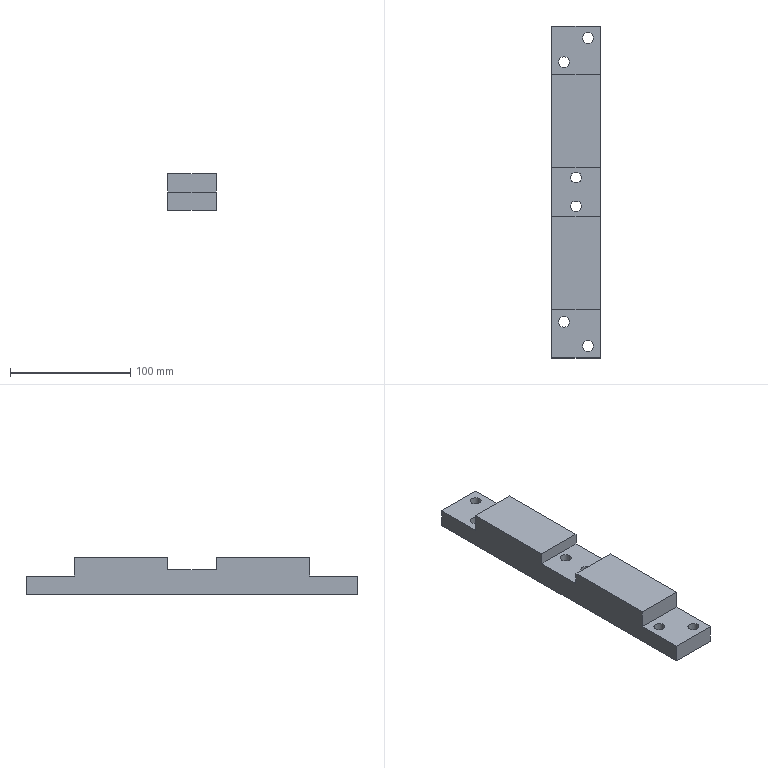Part | NX | features solid 2 | 1 solid | 24 faces | box 40 x 276 x 30 mm | volume 258605 mm3 | plane 16 | cylinder 8 | commonest cylinder face diameters 9 x6 14.5 x2
STEP:
#1=CARTESIAN_POINT('',(3416.5,-108.,-63.5));
#2=VERTEX_POINT('',#1);
#3=CARTESIAN_POINT('',(3421.,-108.,-63.5));
#4=DIRECTION('',(0.,0.,-1.));
#5=DIRECTION('',(-1.,0.,0.));
#6=AXIS2_PLACEMENT_3D('',#3,#4,#5);
#7=CIRCLE('',#6,4.5);
#8=EDGE_CURVE('',#2,#2,#7,.T.);
#9=ORIENTED_EDGE('',*,*,#8,.F.);
#10=EDGE_LOOP('',(#9));
#11=FACE_BOUND('',#10,.T.);
#12=CARTESIAN_POINT('',(3438.25,-12.,-63.5));
#13=VERTEX_POINT('',#12);
#14=CARTESIAN_POINT('',(3431.,-12.,-63.5));
#15=DIRECTION('',(0.,0.,1.));
#16=DIRECTION('',(1.,0.,0.));
#17=AXIS2_PLACEMENT_3D('',#14,#15,#16);
#18=CIRCLE('',#17,7.25);
#19=EDGE_CURVE('',#13,#13,#18,.T.);
#20=ORIENTED_EDGE('',*,*,#19,.T.);
#21=EDGE_LOOP('',(#20));
#22=FACE_BOUND('',#21,.T.);
#23=CARTESIAN_POINT('',(3411.,138.,-63.5));
#24=VERTEX_POINT('',#23);
#25=CARTESIAN_POINT('',(3411.,-138.,-63.5));
#26=VERTEX_POINT('',#25);
#27=CARTESIAN_POINT('',(3411.,0.,-63.5));
#28=DIRECTION('',(0.,-1.,0.));
#29=VECTOR('',#28,1000.);
#30=LINE('',#27,#29);
#31=EDGE_CURVE('',#24,#26,#30,.T.);
#32=ORIENTED_EDGE('',*,*,#31,.F.);
#33=CARTESIAN_POINT('',(3451.,138.,-63.5));
#34=VERTEX_POINT('',#33);
#35=CARTESIAN_POINT('',(3699.,138.,-63.5));
#36=DIRECTION('',(1.,0.,0.));
#37=VECTOR('',#36,1000.);
#38=LINE('',#35,#37);
#39=EDGE_CURVE('',#24,#34,#38,.T.);
#40=ORIENTED_EDGE('',*,*,#39,.T.);
#41=CARTESIAN_POINT('',(3451.,-138.,-63.5));
#42=VERTEX_POINT('',#41);
#43=CARTESIAN_POINT('',(3451.,0.,-63.5));
#44=DIRECTION('',(0.,1.,0.));
#45=VECTOR('',#44,1000.);
#46=LINE('',#43,#45);
#47=EDGE_CURVE('',#42,#34,#46,.T.);
#48=ORIENTED_EDGE('',*,*,#47,.F.);
#49=CARTESIAN_POINT('',(3699.,-138.,-63.5));
#50=DIRECTION('',(1.,0.,0.));
#51=VECTOR('',#50,1000.);
#52=LINE('',#49,#51);
#53=EDGE_CURVE('',#26,#42,#52,.T.);
#54=ORIENTED_EDGE('',*,*,#53,.F.);
#55=EDGE_LOOP('',(#32,#40,#48,#54));
#56=FACE_BOUND('',#55,.T.);
#57=CARTESIAN_POINT('',(3445.5,-128.,-63.5));
#58=VERTEX_POINT('',#57);
#59=CARTESIAN_POINT('',(3441.,-128.,-63.5));
#60=DIRECTION('',(0.,0.,1.));
#61=DIRECTION('',(1.,0.,0.));
#62=AXIS2_PLACEMENT_3D('',#59,#60,#61);
#63=CIRCLE('',#62,4.5);
#64=EDGE_CURVE('',#58,#58,#63,.T.);
#65=ORIENTED_EDGE('',*,*,#64,.T.);
#66=EDGE_LOOP('',(#65));
#67=FACE_BOUND('',#66,.T.);
#68=CARTESIAN_POINT('',(3416.5,108.,-63.5));
#69=VERTEX_POINT('',#68);
#70=CARTESIAN_POINT('',(3421.,108.,-63.5));
#71=DIRECTION('',(0.,0.,1.));
#72=DIRECTION('',(-1.,0.,0.));
#73=AXIS2_PLACEMENT_3D('',#70,#71,#72);
#74=CIRCLE('',#73,4.5);
#75=EDGE_CURVE('',#69,#69,#74,.T.);
#76=ORIENTED_EDGE('',*,*,#75,.T.);
#77=EDGE_LOOP('',(#76));
#78=FACE_BOUND('',#77,.T.);
#79=CARTESIAN_POINT('',(3438.25,12.,-63.5));
#80=VERTEX_POINT('',#79);
#81=CARTESIAN_POINT('',(3431.,12.,-63.5));
#82=DIRECTION('',(0.,0.,-1.));
#83=DIRECTION('',(1.,0.,0.));
#84=AXIS2_PLACEMENT_3D('',#81,#82,#83);
#85=CIRCLE('',#84,7.25);
#86=EDGE_CURVE('',#80,#80,#85,.T.);
#87=ORIENTED_EDGE('',*,*,#86,.F.);
#88=EDGE_LOOP('',(#87));
#89=FACE_BOUND('',#88,.T.);
#90=CARTESIAN_POINT('',(3445.5,128.,-63.5));
#91=VERTEX_POINT('',#90);
#92=CARTESIAN_POINT('',(3441.,128.,-63.5));
#93=DIRECTION('',(0.,0.,-1.));
#94=DIRECTION('',(1.,0.,0.));
#95=AXIS2_PLACEMENT_3D('',#92,#93,#94);
#96=CIRCLE('',#95,4.5);
#97=EDGE_CURVE('',#91,#91,#96,.T.);
#98=ORIENTED_EDGE('',*,*,#97,.F.);
#99=EDGE_LOOP('',(#98));
#100=FACE_BOUND('',#99,.T.);
#101=CARTESIAN_POINT('',(3421.,0.,-63.5));
#102=DIRECTION('',(0.,0.,-1.));
#103=DIRECTION('',(1.,0.,0.));
#104=AXIS2_PLACEMENT_3D('',#101,#102,#103);
#105=PLANE('',#104);
#106=ADVANCED_FACE('',(#11,#22,#56,#67,#78,#89,#100),#105,.T.);
#107=CARTESIAN_POINT('',(3411.,20.,-43.5));
#108=VERTEX_POINT('',#107);
#109=CARTESIAN_POINT('',(3411.,-20.,-43.5));
#110=VERTEX_POINT('',#109);
#111=CARTESIAN_POINT('',(3411.,0.,-43.5));
#112=DIRECTION('',(0.,-1.,0.));
#113=VECTOR('',#112,1000.);
#114=LINE('',#111,#113);
#115=EDGE_CURVE('',#108,#110,#114,.T.);
#116=ORIENTED_EDGE('',*,*,#115,.F.);
#117=CARTESIAN_POINT('',(3411.,20.,-33.5));
#118=VERTEX_POINT('',#117);
#119=CARTESIAN_POINT('',(3411.,20.,-63.5));
#120=DIRECTION('',(0.,0.,1.));
#121=VECTOR('',#120,1000.);
#122=LINE('',#119,#121);
#123=EDGE_CURVE('',#108,#118,#122,.T.);
#124=ORIENTED_EDGE('',*,*,#123,.T.);
#125=CARTESIAN_POINT('',(3411.,98.,-33.5));
#126=VERTEX_POINT('',#125);
#127=CARTESIAN_POINT('',(3411.,0.,-33.5));
#128=DIRECTION('',(0.,-1.,0.));
#129=VECTOR('',#128,1000.);
#130=LINE('',#127,#129);
#131=EDGE_CURVE('',#126,#118,#130,.T.);
#132=ORIENTED_EDGE('',*,*,#131,.F.);
#133=CARTESIAN_POINT('',(3411.,98.,-48.5));
#134=VERTEX_POINT('',#133);
#135=CARTESIAN_POINT('',(3411.,98.,-53.5));
#136=DIRECTION('',(0.,0.,1.));
#137=VECTOR('',#136,1000.);
#138=LINE('',#135,#137);
#139=EDGE_CURVE('',#134,#126,#138,.T.);
#140=ORIENTED_EDGE('',*,*,#139,.F.);
#141=CARTESIAN_POINT('',(3411.,138.,-48.5));
#142=VERTEX_POINT('',#141);
#143=CARTESIAN_POINT('',(3411.,0.,-48.5));
#144=DIRECTION('',(0.,1.,0.));
#145=VECTOR('',#144,1000.);
#146=LINE('',#143,#145);
#147=EDGE_CURVE('',#134,#142,#146,.T.);
#148=ORIENTED_EDGE('',*,*,#147,.T.);
#149=CARTESIAN_POINT('',(3411.,138.,-63.5));
#150=DIRECTION('',(0.,0.,1.));
#151=VECTOR('',#150,1000.);
#152=LINE('',#149,#151);
#153=EDGE_CURVE('',#24,#142,#152,.T.);
#154=ORIENTED_EDGE('',*,*,#153,.F.);
#155=ORIENTED_EDGE('',*,*,#31,.T.);
#156=CARTESIAN_POINT('',(3411.,-138.,-48.5));
#157=VERTEX_POINT('',#156);
#158=CARTESIAN_POINT('',(3411.,-138.,-63.5));
#159=DIRECTION('',(0.,0.,1.));
#160=VECTOR('',#159,1000.);
#161=LINE('',#158,#160);
#162=EDGE_CURVE('',#26,#157,#161,.T.);
#163=ORIENTED_EDGE('',*,*,#162,.T.);
#164=CARTESIAN_POINT('',(3411.,-98.,-48.5));
#165=VERTEX_POINT('',#164);
#166=CARTESIAN_POINT('',(3411.,0.,-48.5));
#167=DIRECTION('',(0.,-1.,0.));
#168=VECTOR('',#167,1000.);
#169=LINE('',#166,#168);
#170=EDGE_CURVE('',#165,#157,#169,.T.);
#171=ORIENTED_EDGE('',*,*,#170,.F.);
#172=CARTESIAN_POINT('',(3411.,-98.,-33.5));
#173=VERTEX_POINT('',#172);
#174=CARTESIAN_POINT('',(3411.,-98.,-53.5));
#175=DIRECTION('',(0.,0.,1.));
#176=VECTOR('',#175,1000.);
#177=LINE('',#174,#176);
#178=EDGE_CURVE('',#165,#173,#177,.T.);
#179=ORIENTED_EDGE('',*,*,#178,.T.);
#180=CARTESIAN_POINT('',(3411.,-20.,-33.5));
#181=VERTEX_POINT('',#180);
#182=CARTESIAN_POINT('',(3411.,0.,-33.5));
#183=DIRECTION('',(0.,1.,0.));
#184=VECTOR('',#183,1000.);
#185=LINE('',#182,#184);
#186=EDGE_CURVE('',#173,#181,#185,.T.);
#187=ORIENTED_EDGE('',*,*,#186,.T.);
#188=CARTESIAN_POINT('',(3411.,-20.,-63.5));
#189=DIRECTION('',(0.,0.,1.));
#190=VECTOR('',#189,1000.);
#191=LINE('',#188,#190);
#192=EDGE_CURVE('',#110,#181,#191,.T.);
#193=ORIENTED_EDGE('',*,*,#192,.F.);
#194=EDGE_LOOP('',(#116,#124,#132,#140,#148,#154,#155,#163,#171,#179,#187,#193));
#195=FACE_BOUND('',#194,.T.);
#196=CARTESIAN_POINT('',(3411.,0.,-63.5));
#197=DIRECTION('',(-1.,0.,0.));
#198=DIRECTION('',(0.,0.,-1.));
#199=AXIS2_PLACEMENT_3D('',#196,#197,#198);
#200=PLANE('',#199);
#201=ADVANCED_FACE('',(#195),#200,.T.);
#202=ORIENTED_EDGE('',*,*,#47,.T.);
#203=CARTESIAN_POINT('',(3451.,138.,-48.5));
#204=VERTEX_POINT('',#203);
#205=CARTESIAN_POINT('',(3451.,138.,-53.5));
#206=DIRECTION('',(0.,0.,1.));
#207=VECTOR('',#206,1000.);
#208=LINE('',#205,#207);
#209=EDGE_CURVE('',#34,#204,#208,.T.);
#210=ORIENTED_EDGE('',*,*,#209,.T.);
#211=CARTESIAN_POINT('',(3451.,98.,-48.5));
#212=VERTEX_POINT('',#211);
#213=CARTESIAN_POINT('',(3451.,0.,-48.5));
#214=DIRECTION('',(0.,-1.,0.));
#215=VECTOR('',#214,1000.);
#216=LINE('',#213,#215);
#217=EDGE_CURVE('',#204,#212,#216,.T.);
#218=ORIENTED_EDGE('',*,*,#217,.T.);
#219=CARTESIAN_POINT('',(3451.,98.,-33.5));
#220=VERTEX_POINT('',#219);
#221=CARTESIAN_POINT('',(3451.,98.,-63.5));
#222=DIRECTION('',(0.,0.,1.));
#223=VECTOR('',#222,1000.);
#224=LINE('',#221,#223);
#225=EDGE_CURVE('',#212,#220,#224,.T.);
#226=ORIENTED_EDGE('',*,*,#225,.T.);
#227=CARTESIAN_POINT('',(3451.,20.,-33.5));
#228=VERTEX_POINT('',#227);
#229=CARTESIAN_POINT('',(3451.,0.,-33.5));
#230=DIRECTION('',(0.,1.,0.));
#231=VECTOR('',#230,1000.);
#232=LINE('',#229,#231);
#233=EDGE_CURVE('',#228,#220,#232,.T.);
#234=ORIENTED_EDGE('',*,*,#233,.F.);
#235=CARTESIAN_POINT('',(3451.,20.,-43.5));
#236=VERTEX_POINT('',#235);
#237=CARTESIAN_POINT('',(3451.,20.,-63.5));
#238=DIRECTION('',(0.,0.,-1.));
#239=VECTOR('',#238,1000.);
#240=LINE('',#237,#239);
#241=EDGE_CURVE('',#228,#236,#240,.T.);
#242=ORIENTED_EDGE('',*,*,#241,.T.);
#243=CARTESIAN_POINT('',(3451.,-20.,-43.5));
#244=VERTEX_POINT('',#243);
#245=CARTESIAN_POINT('',(3451.,0.,-43.5));
#246=DIRECTION('',(0.,1.,0.));
#247=VECTOR('',#246,1000.);
#248=LINE('',#245,#247);
#249=EDGE_CURVE('',#244,#236,#248,.T.);
#250=ORIENTED_EDGE('',*,*,#249,.F.);
#251=CARTESIAN_POINT('',(3451.,-20.,-33.5));
#252=VERTEX_POINT('',#251);
#253=CARTESIAN_POINT('',(3451.,-20.,-63.5));
#254=DIRECTION('',(0.,0.,-1.));
#255=VECTOR('',#254,1000.);
#256=LINE('',#253,#255);
#257=EDGE_CURVE('',#252,#244,#256,.T.);
#258=ORIENTED_EDGE('',*,*,#257,.F.);
#259=CARTESIAN_POINT('',(3451.,-98.,-33.5));
#260=VERTEX_POINT('',#259);
#261=CARTESIAN_POINT('',(3451.,0.,-33.5));
#262=DIRECTION('',(0.,-1.,0.));
#263=VECTOR('',#262,1000.);
#264=LINE('',#261,#263);
#265=EDGE_CURVE('',#252,#260,#264,.T.);
#266=ORIENTED_EDGE('',*,*,#265,.T.);
#267=CARTESIAN_POINT('',(3451.,-98.,-48.5));
#268=VERTEX_POINT('',#267);
#269=CARTESIAN_POINT('',(3451.,-98.,-63.5));
#270=DIRECTION('',(0.,0.,1.));
#271=VECTOR('',#270,1000.);
#272=LINE('',#269,#271);
#273=EDGE_CURVE('',#268,#260,#272,.T.);
#274=ORIENTED_EDGE('',*,*,#273,.F.);
#275=CARTESIAN_POINT('',(3451.,-138.,-48.5));
#276=VERTEX_POINT('',#275);
#277=CARTESIAN_POINT('',(3451.,0.,-48.5));
#278=DIRECTION('',(0.,1.,0.));
#279=VECTOR('',#278,1000.);
#280=LINE('',#277,#279);
#281=EDGE_CURVE('',#276,#268,#280,.T.);
#282=ORIENTED_EDGE('',*,*,#281,.F.);
#283=CARTESIAN_POINT('',(3451.,-138.,-53.5));
#284=DIRECTION('',(0.,0.,1.));
#285=VECTOR('',#284,1000.);
#286=LINE('',#283,#285);
#287=EDGE_CURVE('',#42,#276,#286,.T.);
#288=ORIENTED_EDGE('',*,*,#287,.F.);
#289=EDGE_LOOP('',(#202,#210,#218,#226,#234,#242,#250,#258,#266,#274,#282,#288));
#290=FACE_BOUND('',#289,.T.);
#291=CARTESIAN_POINT('',(3451.,0.,-63.5));
#292=DIRECTION('',(1.,0.,0.));
#293=DIRECTION('',(0.,0.,1.));
#294=AXIS2_PLACEMENT_3D('',#291,#292,#293);
#295=PLANE('',#294);
#296=ADVANCED_FACE('',(#290),#295,.T.);
#297=CARTESIAN_POINT('',(3435.5,-12.,-43.5));
#298=VERTEX_POINT('',#297);
#299=CARTESIAN_POINT('',(3431.,-12.,-43.5));
#300=DIRECTION('',(0.,0.,-1.));
#301=DIRECTION('',(1.,0.,0.));
#302=AXIS2_PLACEMENT_3D('',#299,#300,#301);
#303=CIRCLE('',#302,4.5);
#304=EDGE_CURVE('',#298,#298,#303,.T.);
#305=ORIENTED_EDGE('',*,*,#304,.T.);
#306=EDGE_LOOP('',(#305));
#307=FACE_BOUND('',#306,.T.);
#308=ORIENTED_EDGE('',*,*,#249,.T.);
#309=CARTESIAN_POINT('',(2860.,20.,-43.5));
#310=DIRECTION('',(-1.,0.,0.));
#311=VECTOR('',#310,1000.);
#312=LINE('',#309,#311);
#313=EDGE_CURVE('',#236,#108,#312,.T.);
#314=ORIENTED_EDGE('',*,*,#313,.T.);
#315=ORIENTED_EDGE('',*,*,#115,.T.);
#316=CARTESIAN_POINT('',(2860.,-20.,-43.5));
#317=DIRECTION('',(-1.,0.,0.));
#318=VECTOR('',#317,1000.);
#319=LINE('',#316,#318);
#320=EDGE_CURVE('',#244,#110,#319,.T.);
#321=ORIENTED_EDGE('',*,*,#320,.F.);
#322=EDGE_LOOP('',(#308,#314,#315,#321));
#323=FACE_BOUND('',#322,.T.);
#324=CARTESIAN_POINT('',(3435.5,12.,-43.5));
#325=VERTEX_POINT('',#324);
#326=CARTESIAN_POINT('',(3431.,12.,-43.5));
#327=DIRECTION('',(0.,0.,1.));
#328=DIRECTION('',(1.,0.,0.));
#329=AXIS2_PLACEMENT_3D('',#326,#327,#328);
#330=CIRCLE('',#329,4.5);
#331=EDGE_CURVE('',#325,#325,#330,.T.);
#332=ORIENTED_EDGE('',*,*,#331,.F.);
#333=EDGE_LOOP('',(#332));
#334=FACE_BOUND('',#333,.T.);
#335=CARTESIAN_POINT('',(2544.879,0.,-43.5));
#336=DIRECTION('',(0.,0.,1.));
#337=DIRECTION('',(-1.,0.,0.));
#338=AXIS2_PLACEMENT_3D('',#335,#336,#337);
#339=PLANE('',#338);
#340=ADVANCED_FACE('',(#307,#323,#334),#339,.T.);
#341=CARTESIAN_POINT('',(3421.,-20.,-33.5));
#342=DIRECTION('',(1.,0.,0.));
#343=VECTOR('',#342,1000.);
#344=LINE('',#341,#343);
#345=EDGE_CURVE('',#181,#252,#344,.T.);
#346=ORIENTED_EDGE('',*,*,#345,.F.);
#347=ORIENTED_EDGE('',*,*,#186,.F.);
#348=CARTESIAN_POINT('',(3699.,-98.,-33.5));
#349=DIRECTION('',(1.,0.,0.));
#350=VECTOR('',#349,1000.);
#351=LINE('',#348,#350);
#352=EDGE_CURVE('',#173,#260,#351,.T.);
#353=ORIENTED_EDGE('',*,*,#352,.T.);
#354=ORIENTED_EDGE('',*,*,#265,.F.);
#355=EDGE_LOOP('',(#346,#347,#353,#354));
#356=FACE_BOUND('',#355,.T.);
#357=CARTESIAN_POINT('',(3421.,0.,-33.5));
#358=DIRECTION('',(0.,0.,1.));
#359=DIRECTION('',(-1.,0.,0.));
#360=AXIS2_PLACEMENT_3D('',#357,#358,#359);
#361=PLANE('',#360);
#362=ADVANCED_FACE('',(#356),#361,.T.);
#363=CARTESIAN_POINT('',(3699.,-138.,-48.5));
#364=DIRECTION('',(1.,0.,0.));
#365=VECTOR('',#364,1000.);
#366=LINE('',#363,#365);
#367=EDGE_CURVE('',#157,#276,#366,.T.);
#368=ORIENTED_EDGE('',*,*,#367,.F.);
#369=ORIENTED_EDGE('',*,*,#162,.F.);
#370=ORIENTED_EDGE('',*,*,#53,.T.);
#371=ORIENTED_EDGE('',*,*,#287,.T.);
#372=EDGE_LOOP('',(#368,#369,#370,#371));
#373=FACE_BOUND('',#372,.T.);
#374=CARTESIAN_POINT('',(3699.,-138.,-53.5));
#375=DIRECTION('',(0.,-1.,0.));
#376=DIRECTION('',(0.,0.,1.));
#377=AXIS2_PLACEMENT_3D('',#374,#375,#376);
#378=PLANE('',#377);
#379=ADVANCED_FACE('',(#373),#378,.T.);
#380=CARTESIAN_POINT('',(3445.5,-128.,-48.5));
#381=VERTEX_POINT('',#380);
#382=CARTESIAN_POINT('',(3441.,-128.,-48.5));
#383=DIRECTION('',(0.,0.,1.));
#384=DIRECTION('',(1.,0.,0.));
#385=AXIS2_PLACEMENT_3D('',#382,#383,#384);
#386=CIRCLE('',#385,4.5);
#387=EDGE_CURVE('',#381,#381,#386,.T.);
#388=ORIENTED_EDGE('',*,*,#387,.F.);
#389=EDGE_LOOP('',(#388));
#390=FACE_BOUND('',#389,.T.);
#391=CARTESIAN_POINT('',(3425.5,-108.,-48.5));
#392=VERTEX_POINT('',#391);
#393=CARTESIAN_POINT('',(3421.,-108.,-48.5));
#394=DIRECTION('',(0.,0.,1.));
#395=DIRECTION('',(1.,0.,0.));
#396=AXIS2_PLACEMENT_3D('',#393,#394,#395);
#397=CIRCLE('',#396,4.5);
#398=EDGE_CURVE('',#392,#392,#397,.T.);
#399=ORIENTED_EDGE('',*,*,#398,.F.);
#400=EDGE_LOOP('',(#399));
#401=FACE_BOUND('',#400,.T.);
#402=ORIENTED_EDGE('',*,*,#281,.T.);
#403=CARTESIAN_POINT('',(3699.,-98.,-48.5));
#404=DIRECTION('',(-1.,0.,0.));
#405=VECTOR('',#404,1000.);
#406=LINE('',#403,#405);
#407=EDGE_CURVE('',#268,#165,#406,.T.);
#408=ORIENTED_EDGE('',*,*,#407,.T.);
#409=ORIENTED_EDGE('',*,*,#170,.T.);
#410=ORIENTED_EDGE('',*,*,#367,.T.);
#411=EDGE_LOOP('',(#402,#408,#409,#410));
#412=FACE_BOUND('',#411,.T.);
#413=CARTESIAN_POINT('',(3411.,-138.,-48.5));
#414=DIRECTION('',(0.,0.,1.));
#415=DIRECTION('',(-1.,0.,0.));
#416=AXIS2_PLACEMENT_3D('',#413,#414,#415);
#417=PLANE('',#416);
#418=ADVANCED_FACE('',(#390,#401,#412),#417,.T.);
#419=ORIENTED_EDGE('',*,*,#273,.T.);
#420=ORIENTED_EDGE('',*,*,#352,.F.);
#421=ORIENTED_EDGE('',*,*,#178,.F.);
#422=ORIENTED_EDGE('',*,*,#407,.F.);
#423=EDGE_LOOP('',(#419,#420,#421,#422));
#424=FACE_BOUND('',#423,.T.);
#425=CARTESIAN_POINT('',(3699.,-98.,-53.5));
#426=DIRECTION('',(0.,1.,0.));
#427=DIRECTION('',(0.,0.,-1.));
#428=AXIS2_PLACEMENT_3D('',#425,#426,#427);
#429=PLANE('',#428);
#430=ADVANCED_FACE('',(#424),#429,.F.);
#431=ORIENTED_EDGE('',*,*,#192,.T.);
#432=ORIENTED_EDGE('',*,*,#345,.T.);
#433=ORIENTED_EDGE('',*,*,#257,.T.);
#434=ORIENTED_EDGE('',*,*,#320,.T.);
#435=EDGE_LOOP('',(#431,#432,#433,#434));
#436=FACE_BOUND('',#435,.T.);
#437=CARTESIAN_POINT('',(2860.,-20.,-23.5));
#438=DIRECTION('',(0.,-1.,0.));
#439=DIRECTION('',(0.,0.,1.));
#440=AXIS2_PLACEMENT_3D('',#437,#438,#439);
#441=PLANE('',#440);
#442=ADVANCED_FACE('',(#436),#441,.F.);
#443=CARTESIAN_POINT('',(3435.5,-12.,-52.5));
#444=VERTEX_POINT('',#443);
#445=CARTESIAN_POINT('',(3431.,-12.,-52.5));
#446=DIRECTION('',(0.,0.,1.));
#447=DIRECTION('',(1.,0.,0.));
#448=AXIS2_PLACEMENT_3D('',#445,#446,#447);
#449=CIRCLE('',#448,4.5);
#450=EDGE_CURVE('',#444,#444,#449,.T.);
#451=ORIENTED_EDGE('',*,*,#450,.F.);
#452=EDGE_LOOP('',(#451));
#453=FACE_BOUND('',#452,.T.);
#454=ORIENTED_EDGE('',*,*,#304,.F.);
#455=EDGE_LOOP('',(#454));
#456=FACE_BOUND('',#455,.T.);
#457=CARTESIAN_POINT('',(3431.,-12.,-63.5));
#458=DIRECTION('',(0.,0.,1.));
#459=DIRECTION('',(-1.,0.,0.));
#460=AXIS2_PLACEMENT_3D('',#457,#458,#459);
#461=CYLINDRICAL_SURFACE('',#460,4.5);
#462=ADVANCED_FACE('',(#453,#456),#461,.F.);
#463=ORIENTED_EDGE('',*,*,#450,.T.);
#464=EDGE_LOOP('',(#463));
#465=FACE_BOUND('',#464,.T.);
#466=CARTESIAN_POINT('',(3438.25,-12.,-52.5));
#467=VERTEX_POINT('',#466);
#468=CARTESIAN_POINT('',(3431.,-12.,-52.5));
#469=DIRECTION('',(0.,0.,1.));
#470=DIRECTION('',(1.,0.,0.));
#471=AXIS2_PLACEMENT_3D('',#468,#469,#470);
#472=CIRCLE('',#471,7.25);
#473=EDGE_CURVE('',#467,#467,#472,.T.);
#474=ORIENTED_EDGE('',*,*,#473,.F.);
#475=EDGE_LOOP('',(#474));
#476=FACE_BOUND('',#475,.T.);
#477=CARTESIAN_POINT('',(3431.,-12.,-52.5));
#478=DIRECTION('',(0.,0.,1.));
#479=DIRECTION('',(-1.,0.,0.));
#480=AXIS2_PLACEMENT_3D('',#477,#478,#479);
#481=PLANE('',#480);
#482=ADVANCED_FACE('',(#465,#476),#481,.F.);
#483=ORIENTED_EDGE('',*,*,#473,.T.);
#484=EDGE_LOOP('',(#483));
#485=FACE_BOUND('',#484,.T.);
#486=ORIENTED_EDGE('',*,*,#19,.F.);
#487=EDGE_LOOP('',(#486));
#488=FACE_BOUND('',#487,.T.);
#489=CARTESIAN_POINT('',(3431.,-12.,-63.5));
#490=DIRECTION('',(0.,0.,1.));
#491=DIRECTION('',(-1.,0.,0.));
#492=AXIS2_PLACEMENT_3D('',#489,#490,#491);
#493=CYLINDRICAL_SURFACE('',#492,7.25);
#494=ADVANCED_FACE('',(#485,#488),#493,.F.);
#495=ORIENTED_EDGE('',*,*,#398,.T.);
#496=EDGE_LOOP('',(#495));
#497=FACE_BOUND('',#496,.T.);
#498=ORIENTED_EDGE('',*,*,#8,.T.);
#499=EDGE_LOOP('',(#498));
#500=FACE_BOUND('',#499,.T.);
#501=CARTESIAN_POINT('',(3421.,-108.,-74.5));
#502=DIRECTION('',(0.,0.,1.));
#503=DIRECTION('',(-1.,0.,0.));
#504=AXIS2_PLACEMENT_3D('',#501,#502,#503);
#505=CYLINDRICAL_SURFACE('',#504,4.5);
#506=ADVANCED_FACE('',(#497,#500),#505,.F.);
#507=ORIENTED_EDGE('',*,*,#387,.T.);
#508=EDGE_LOOP('',(#507));
#509=FACE_BOUND('',#508,.T.);
#510=ORIENTED_EDGE('',*,*,#64,.F.);
#511=EDGE_LOOP('',(#510));
#512=FACE_BOUND('',#511,.T.);
#513=CARTESIAN_POINT('',(3441.,-128.,-74.5));
#514=DIRECTION('',(0.,0.,1.));
#515=DIRECTION('',(1.,0.,0.));
#516=AXIS2_PLACEMENT_3D('',#513,#514,#515);
#517=CYLINDRICAL_SURFACE('',#516,4.5);
#518=ADVANCED_FACE('',(#509,#512),#517,.F.);
#519=CARTESIAN_POINT('',(3421.,20.,-33.5));
#520=DIRECTION('',(1.,0.,0.));
#521=VECTOR('',#520,1000.);
#522=LINE('',#519,#521);
#523=EDGE_CURVE('',#118,#228,#522,.T.);
#524=ORIENTED_EDGE('',*,*,#523,.T.);
#525=ORIENTED_EDGE('',*,*,#233,.T.);
#526=CARTESIAN_POINT('',(3699.,98.,-33.5));
#527=DIRECTION('',(1.,0.,0.));
#528=VECTOR('',#527,1000.);
#529=LINE('',#526,#528);
#530=EDGE_CURVE('',#126,#220,#529,.T.);
#531=ORIENTED_EDGE('',*,*,#530,.F.);
#532=ORIENTED_EDGE('',*,*,#131,.T.);
#533=EDGE_LOOP('',(#524,#525,#531,#532));
#534=FACE_BOUND('',#533,.T.);
#535=CARTESIAN_POINT('',(3421.,0.,-33.5));
#536=DIRECTION('',(0.,0.,1.));
#537=DIRECTION('',(-1.,0.,0.));
#538=AXIS2_PLACEMENT_3D('',#535,#536,#537);
#539=PLANE('',#538);
#540=ADVANCED_FACE('',(#534),#539,.T.);
#541=CARTESIAN_POINT('',(3699.,138.,-48.5));
#542=DIRECTION('',(1.,0.,0.));
#543=VECTOR('',#542,1000.);
#544=LINE('',#541,#543);
#545=EDGE_CURVE('',#142,#204,#544,.T.);
#546=ORIENTED_EDGE('',*,*,#545,.T.);
#547=ORIENTED_EDGE('',*,*,#209,.F.);
#548=ORIENTED_EDGE('',*,*,#39,.F.);
#549=ORIENTED_EDGE('',*,*,#153,.T.);
#550=EDGE_LOOP('',(#546,#547,#548,#549));
#551=FACE_BOUND('',#550,.T.);
#552=CARTESIAN_POINT('',(3699.,138.,-53.5));
#553=DIRECTION('',(0.,1.,0.));
#554=DIRECTION('',(0.,0.,1.));
#555=AXIS2_PLACEMENT_3D('',#552,#553,#554);
#556=PLANE('',#555);
#557=ADVANCED_FACE('',(#551),#556,.T.);
#558=CARTESIAN_POINT('',(3445.5,128.,-48.5));
#559=VERTEX_POINT('',#558);
#560=CARTESIAN_POINT('',(3441.,128.,-48.5));
#561=DIRECTION('',(0.,0.,-1.));
#562=DIRECTION('',(1.,0.,0.));
#563=AXIS2_PLACEMENT_3D('',#560,#561,#562);
#564=CIRCLE('',#563,4.5);
#565=EDGE_CURVE('',#559,#559,#564,.T.);
#566=ORIENTED_EDGE('',*,*,#565,.T.);
#567=EDGE_LOOP('',(#566));
#568=FACE_BOUND('',#567,.T.);
#569=CARTESIAN_POINT('',(3425.5,108.,-48.5));
#570=VERTEX_POINT('',#569);
#571=CARTESIAN_POINT('',(3421.,108.,-48.5));
#572=DIRECTION('',(0.,0.,-1.));
#573=DIRECTION('',(1.,0.,0.));
#574=AXIS2_PLACEMENT_3D('',#571,#572,#573);
#575=CIRCLE('',#574,4.5);
#576=EDGE_CURVE('',#570,#570,#575,.T.);
#577=ORIENTED_EDGE('',*,*,#576,.T.);
#578=EDGE_LOOP('',(#577));
#579=FACE_BOUND('',#578,.T.);
#580=ORIENTED_EDGE('',*,*,#217,.F.);
#581=ORIENTED_EDGE('',*,*,#545,.F.);
#582=ORIENTED_EDGE('',*,*,#147,.F.);
#583=CARTESIAN_POINT('',(3699.,98.,-48.5));
#584=DIRECTION('',(-1.,0.,0.));
#585=VECTOR('',#584,1000.);
#586=LINE('',#583,#585);
#587=EDGE_CURVE('',#212,#134,#586,.T.);
#588=ORIENTED_EDGE('',*,*,#587,.F.);
#589=EDGE_LOOP('',(#580,#581,#582,#588));
#590=FACE_BOUND('',#589,.T.);
#591=CARTESIAN_POINT('',(3411.,138.,-48.5));
#592=DIRECTION('',(0.,0.,1.));
#593=DIRECTION('',(-1.,0.,0.));
#594=AXIS2_PLACEMENT_3D('',#591,#592,#593);
#595=PLANE('',#594);
#596=ADVANCED_FACE('',(#568,#579,#590),#595,.T.);
#597=ORIENTED_EDGE('',*,*,#225,.F.);
#598=ORIENTED_EDGE('',*,*,#587,.T.);
#599=ORIENTED_EDGE('',*,*,#139,.T.);
#600=ORIENTED_EDGE('',*,*,#530,.T.);
#601=EDGE_LOOP('',(#597,#598,#599,#600));
#602=FACE_BOUND('',#601,.T.);
#603=CARTESIAN_POINT('',(3699.,98.,-53.5));
#604=DIRECTION('',(0.,-1.,0.));
#605=DIRECTION('',(0.,0.,-1.));
#606=AXIS2_PLACEMENT_3D('',#603,#604,#605);
#607=PLANE('',#606);
#608=ADVANCED_FACE('',(#602),#607,.F.);
#609=ORIENTED_EDGE('',*,*,#123,.F.);
#610=ORIENTED_EDGE('',*,*,#313,.F.);
#611=ORIENTED_EDGE('',*,*,#241,.F.);
#612=ORIENTED_EDGE('',*,*,#523,.F.);
#613=EDGE_LOOP('',(#609,#610,#611,#612));
#614=FACE_BOUND('',#613,.T.);
#615=CARTESIAN_POINT('',(2860.,20.,-23.5));
#616=DIRECTION('',(0.,1.,0.));
#617=DIRECTION('',(0.,0.,1.));
#618=AXIS2_PLACEMENT_3D('',#615,#616,#617);
#619=PLANE('',#618);
#620=ADVANCED_FACE('',(#614),#619,.F.);
#621=CARTESIAN_POINT('',(3435.5,12.,-52.5));
#622=VERTEX_POINT('',#621);
#623=CARTESIAN_POINT('',(3431.,12.,-52.5));
#624=DIRECTION('',(0.,0.,-1.));
#625=DIRECTION('',(1.,0.,0.));
#626=AXIS2_PLACEMENT_3D('',#623,#624,#625);
#627=CIRCLE('',#626,4.5);
#628=EDGE_CURVE('',#622,#622,#627,.T.);
#629=ORIENTED_EDGE('',*,*,#628,.T.);
#630=EDGE_LOOP('',(#629));
#631=FACE_BOUND('',#630,.T.);
#632=ORIENTED_EDGE('',*,*,#331,.T.);
#633=EDGE_LOOP('',(#632));
#634=FACE_BOUND('',#633,.T.);
#635=CARTESIAN_POINT('',(3431.,12.,-63.5));
#636=DIRECTION('',(0.,0.,1.));
#637=DIRECTION('',(-1.,0.,0.));
#638=AXIS2_PLACEMENT_3D('',#635,#636,#637);
#639=CYLINDRICAL_SURFACE('',#638,4.5);
#640=ADVANCED_FACE('',(#631,#634),#639,.F.);
#641=ORIENTED_EDGE('',*,*,#628,.F.);
#642=EDGE_LOOP('',(#641));
#643=FACE_BOUND('',#642,.T.);
#644=CARTESIAN_POINT('',(3438.25,12.,-52.5));
#645=VERTEX_POINT('',#644);
#646=CARTESIAN_POINT('',(3431.,12.,-52.5));
#647=DIRECTION('',(0.,0.,-1.));
#648=DIRECTION('',(1.,0.,0.));
#649=AXIS2_PLACEMENT_3D('',#646,#647,#648);
#650=CIRCLE('',#649,7.25);
#651=EDGE_CURVE('',#645,#645,#650,.T.);
#652=ORIENTED_EDGE('',*,*,#651,.T.);
#653=EDGE_LOOP('',(#652));
#654=FACE_BOUND('',#653,.T.);
#655=CARTESIAN_POINT('',(3431.,12.,-52.5));
#656=DIRECTION('',(0.,0.,1.));
#657=DIRECTION('',(-1.,0.,0.));
#658=AXIS2_PLACEMENT_3D('',#655,#656,#657);
#659=PLANE('',#658);
#660=ADVANCED_FACE('',(#643,#654),#659,.F.);
#661=ORIENTED_EDGE('',*,*,#651,.F.);
#662=EDGE_LOOP('',(#661));
#663=FACE_BOUND('',#662,.T.);
#664=ORIENTED_EDGE('',*,*,#86,.T.);
#665=EDGE_LOOP('',(#664));
#666=FACE_BOUND('',#665,.T.);
#667=CARTESIAN_POINT('',(3431.,12.,-63.5));
#668=DIRECTION('',(0.,0.,1.));
#669=DIRECTION('',(-1.,0.,0.));
#670=AXIS2_PLACEMENT_3D('',#667,#668,#669);
#671=CYLINDRICAL_SURFACE('',#670,7.25);
#672=ADVANCED_FACE('',(#663,#666),#671,.F.);
#673=ORIENTED_EDGE('',*,*,#576,.F.);
#674=EDGE_LOOP('',(#673));
#675=FACE_BOUND('',#674,.T.);
#676=ORIENTED_EDGE('',*,*,#75,.F.);
#677=EDGE_LOOP('',(#676));
#678=FACE_BOUND('',#677,.T.);
#679=CARTESIAN_POINT('',(3421.,108.,-74.5));
#680=DIRECTION('',(0.,0.,1.));
#681=DIRECTION('',(-1.,0.,0.));
#682=AXIS2_PLACEMENT_3D('',#679,#680,#681);
#683=CYLINDRICAL_SURFACE('',#682,4.5);
#684=ADVANCED_FACE('',(#675,#678),#683,.F.);
#685=ORIENTED_EDGE('',*,*,#565,.F.);
#686=EDGE_LOOP('',(#685));
#687=FACE_BOUND('',#686,.T.);
#688=ORIENTED_EDGE('',*,*,#97,.T.);
#689=EDGE_LOOP('',(#688));
#690=FACE_BOUND('',#689,.T.);
#691=CARTESIAN_POINT('',(3441.,128.,-74.5));
#692=DIRECTION('',(0.,0.,1.));
#693=DIRECTION('',(1.,0.,0.));
#694=AXIS2_PLACEMENT_3D('',#691,#692,#693);
#695=CYLINDRICAL_SURFACE('',#694,4.5);
#696=ADVANCED_FACE('',(#687,#690),#695,.F.);
#697=CLOSED_SHELL('',(#106,#201,#296,#340,#362,#379,#418,#430,#442,#462,#482,#494,#506,#518,#540,#557,#596,#608,#620,#640,#660,#672,#684,#696));
#698=MANIFOLD_SOLID_BREP('',#697);
#699=(LENGTH_UNIT()NAMED_UNIT(*)SI_UNIT(.MILLI.,.METRE.));
#700=UNCERTAINTY_MEASURE_WITH_UNIT(LENGTH_MEASURE(0.00001),#699,'','');
#701=(NAMED_UNIT(*)PLANE_ANGLE_UNIT()SI_UNIT($,.RADIAN.));
#702=(NAMED_UNIT(*)SI_UNIT($,.STERADIAN.)SOLID_ANGLE_UNIT());
#703=(GEOMETRIC_REPRESENTATION_CONTEXT(3)GLOBAL_UNCERTAINTY_ASSIGNED_CONTEXT((#700))GLOBAL_UNIT_ASSIGNED_CONTEXT((#699,#701,#702))REPRESENTATION_CONTEXT('',''));
#704=ADVANCED_BREP_SHAPE_REPRESENTATION('',(#698),#703);